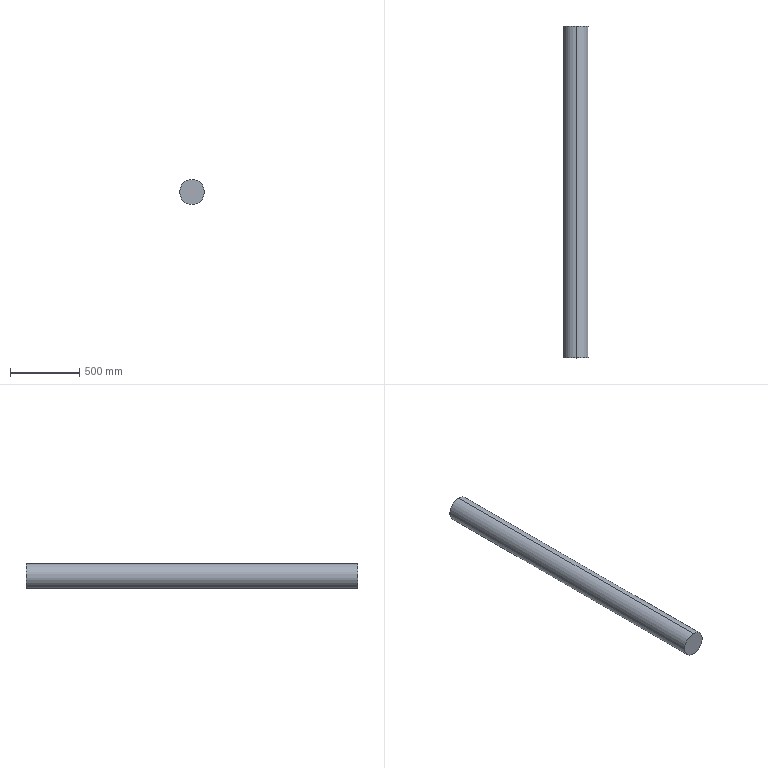Part | SolidWorks | features Extrusion 1 | 1 solid | 4 faces | box 180 x 2400 x 180 mm | volume 61072561 mm3 | cylinder 2 | plane 2 | commonest cylinder face diameters 180 x2
STEP:
#1=CARTESIAN_POINT('',(0.,2400.,90.));
#2=VERTEX_POINT('',#1);
#3=CARTESIAN_POINT('',(0.,2400.,-90.));
#4=VERTEX_POINT('',#3);
#5=CARTESIAN_POINT('',(0.,2400.,0.));
#6=DIRECTION('',(0.,1.,0.));
#7=DIRECTION('',(0.,0.,1.));
#8=AXIS2_PLACEMENT_3D('',#5,#6,#7);
#9=CIRCLE('',#8,90.);
#10=EDGE_CURVE('',#2,#4,#9,.T.);
#11=ORIENTED_EDGE('',*,*,#10,.F.);
#12=CARTESIAN_POINT('',(0.,0.,90.));
#13=VERTEX_POINT('',#12);
#14=CARTESIAN_POINT('',(0.,2400.,90.));
#15=DIRECTION('',(0.,-1.,0.));
#16=VECTOR('',#15,1000.);
#17=LINE('',#14,#16);
#18=EDGE_CURVE('',#2,#13,#17,.T.);
#19=ORIENTED_EDGE('',*,*,#18,.T.);
#20=CARTESIAN_POINT('',(0.,0.,-90.));
#21=VERTEX_POINT('',#20);
#22=CARTESIAN_POINT('',(0.,0.,0.));
#23=DIRECTION('',(0.,1.,0.));
#24=DIRECTION('',(0.,0.,1.));
#25=AXIS2_PLACEMENT_3D('',#22,#23,#24);
#26=CIRCLE('',#25,90.);
#27=EDGE_CURVE('',#13,#21,#26,.T.);
#28=ORIENTED_EDGE('',*,*,#27,.T.);
#29=CARTESIAN_POINT('',(0.,2400.,-90.));
#30=DIRECTION('',(0.,-1.,0.));
#31=VECTOR('',#30,1000.);
#32=LINE('',#29,#31);
#33=EDGE_CURVE('',#4,#21,#32,.T.);
#34=ORIENTED_EDGE('',*,*,#33,.F.);
#35=EDGE_LOOP('',(#11,#19,#28,#34));
#36=FACE_OUTER_BOUND('',#35,.T.);
#37=CARTESIAN_POINT('',(0.,2400.,0.));
#38=DIRECTION('',(0.,-1.,0.));
#39=DIRECTION('',(0.,0.,-1.));
#40=AXIS2_PLACEMENT_3D('',#37,#38,#39);
#41=CYLINDRICAL_SURFACE('',#40,90.);
#42=ADVANCED_FACE('',(#36),#41,.T.);
#43=ORIENTED_EDGE('',*,*,#18,.F.);
#44=CARTESIAN_POINT('',(0.,2400.,0.));
#45=DIRECTION('',(0.,1.,0.));
#46=DIRECTION('',(0.,0.,1.));
#47=AXIS2_PLACEMENT_3D('',#44,#45,#46);
#48=CIRCLE('',#47,90.);
#49=EDGE_CURVE('',#4,#2,#48,.T.);
#50=ORIENTED_EDGE('',*,*,#49,.F.);
#51=ORIENTED_EDGE('',*,*,#33,.T.);
#52=CARTESIAN_POINT('',(0.,0.,0.));
#53=DIRECTION('',(0.,1.,0.));
#54=DIRECTION('',(0.,0.,1.));
#55=AXIS2_PLACEMENT_3D('',#52,#53,#54);
#56=CIRCLE('',#55,90.);
#57=EDGE_CURVE('',#21,#13,#56,.T.);
#58=ORIENTED_EDGE('',*,*,#57,.T.);
#59=EDGE_LOOP('',(#43,#50,#51,#58));
#60=FACE_OUTER_BOUND('',#59,.T.);
#61=CARTESIAN_POINT('',(0.,2400.,0.));
#62=DIRECTION('',(0.,-1.,0.));
#63=DIRECTION('',(0.,0.,-1.));
#64=AXIS2_PLACEMENT_3D('',#61,#62,#63);
#65=CYLINDRICAL_SURFACE('',#64,90.);
#66=ADVANCED_FACE('',(#60),#65,.T.);
#67=ORIENTED_EDGE('',*,*,#49,.T.);
#68=ORIENTED_EDGE('',*,*,#10,.T.);
#69=EDGE_LOOP('',(#67,#68));
#70=FACE_OUTER_BOUND('',#69,.T.);
#71=CARTESIAN_POINT('',(0.,2400.,0.));
#72=DIRECTION('',(0.,1.,0.));
#73=DIRECTION('',(0.,0.,1.));
#74=AXIS2_PLACEMENT_3D('',#71,#72,#73);
#75=PLANE('',#74);
#76=ADVANCED_FACE('',(#70),#75,.T.);
#77=ORIENTED_EDGE('',*,*,#57,.F.);
#78=ORIENTED_EDGE('',*,*,#27,.F.);
#79=EDGE_LOOP('',(#77,#78));
#80=FACE_OUTER_BOUND('',#79,.T.);
#81=CARTESIAN_POINT('',(0.,0.,0.));
#82=DIRECTION('',(0.,1.,0.));
#83=DIRECTION('',(0.,0.,1.));
#84=AXIS2_PLACEMENT_3D('',#81,#82,#83);
#85=PLANE('',#84);
#86=ADVANCED_FACE('',(#80),#85,.F.);
#87=CLOSED_SHELL('',(#42,#66,#76,#86));
#88=MANIFOLD_SOLID_BREP('',#87);
#89=CARTESIAN_POINT('',(0.,0.,0.));
#90=DIRECTION('',(0.,0.,1.));
#91=DIRECTION('',(1.,0.,0.));
#92=AXIS2_PLACEMENT_3D('',#89,#90,#91);
#93=(LENGTH_UNIT()NAMED_UNIT(*)SI_UNIT(.MILLI.,.METRE.));
#94=UNCERTAINTY_MEASURE_WITH_UNIT(LENGTH_MEASURE(0.00001),#93,'','');
#95=(NAMED_UNIT(*)PLANE_ANGLE_UNIT()SI_UNIT($,.RADIAN.));
#96=(NAMED_UNIT(*)SI_UNIT($,.STERADIAN.)SOLID_ANGLE_UNIT());
#97=(GEOMETRIC_REPRESENTATION_CONTEXT(3)GLOBAL_UNCERTAINTY_ASSIGNED_CONTEXT((#94))GLOBAL_UNIT_ASSIGNED_CONTEXT((#93,#95,#96))REPRESENTATION_CONTEXT('',''));
#98=ADVANCED_BREP_SHAPE_REPRESENTATION('',(#88,#92),#97);